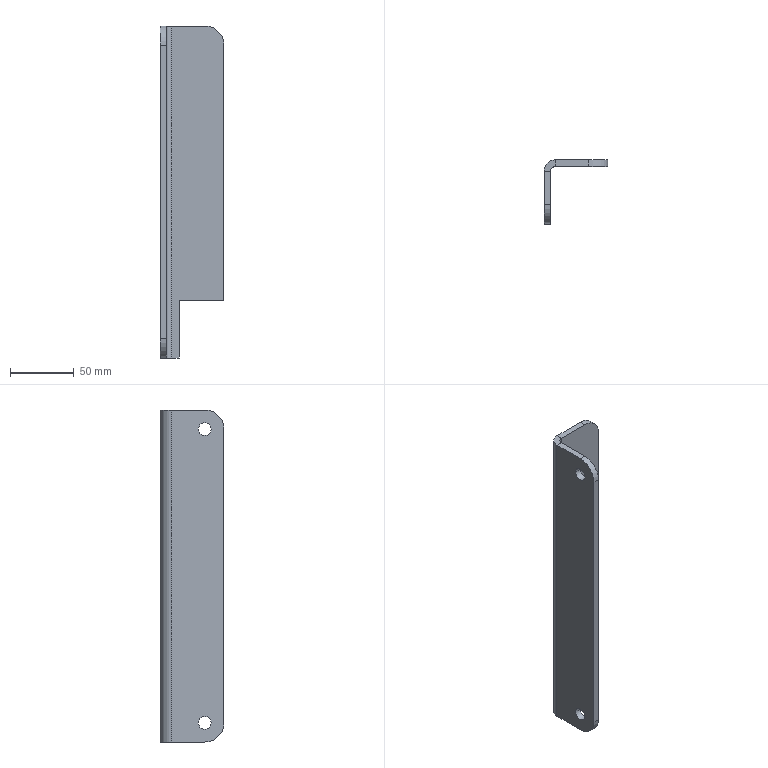Part | STEP file | BCC3 H16_17 | 1 solid | 23 faces | box 50 x 50 x 260 mm | volume 110489 mm3 | plane 14 | cylinder 9 | commonest cylinder face diameters 10 x4 30 x3 8 x1 18 x1